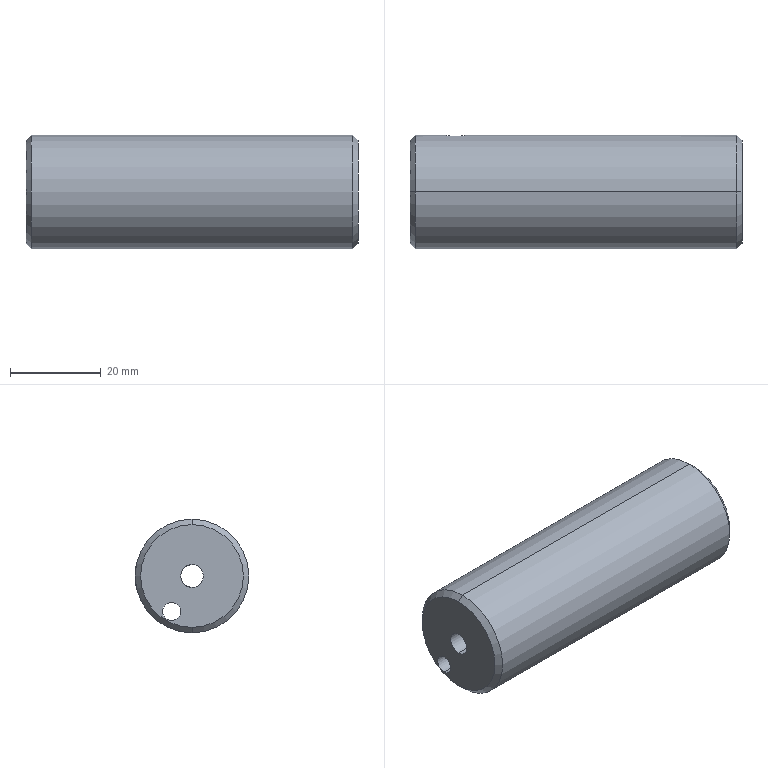Part | NX | features BREP 1 | 1 solid | 15 faces | box 73 x 25 x 25 mm | volume 33171 mm3 | cylinder 9 | cone 4 | plane 2 | commonest cylinder face diameters 5 x5 4 x2 25 x2
STEP:
#1=CARTESIAN_POINT('',(762.255,39.549,-64.084));
#2=VERTEX_POINT('',#1);
#3=CARTESIAN_POINT('',(763.455,39.549,-62.884));
#4=VERTEX_POINT('',#3);
#5=CARTESIAN_POINT('',(762.255,39.549,-64.084));
#6=DIRECTION('',(0.7071,0.,0.7071));
#7=VECTOR('',#6,1000.);
#8=LINE('',#5,#7);
#9=EDGE_CURVE('',#2,#4,#8,.T.);
#10=ORIENTED_EDGE('',*,*,#9,.T.);
#11=CARTESIAN_POINT('',(763.455,39.549,-40.284));
#12=VERTEX_POINT('',#11);
#13=CARTESIAN_POINT('',(763.455,39.549,-51.584));
#14=DIRECTION('',(1.,0.,0.));
#15=DIRECTION('',(0.,0.,1.));
#16=AXIS2_PLACEMENT_3D('',#13,#14,#15);
#17=CIRCLE('',#16,11.3);
#18=EDGE_CURVE('',#12,#4,#17,.T.);
#19=ORIENTED_EDGE('',*,*,#18,.F.);
#20=CARTESIAN_POINT('',(762.255,39.549,-39.084));
#21=VERTEX_POINT('',#20);
#22=CARTESIAN_POINT('',(762.255,39.549,-39.084));
#23=DIRECTION('',(0.7071,0.,-0.7071));
#24=VECTOR('',#23,1000.);
#25=LINE('',#22,#24);
#26=EDGE_CURVE('',#21,#12,#25,.T.);
#27=ORIENTED_EDGE('',*,*,#26,.F.);
#28=CARTESIAN_POINT('',(762.255,39.549,-51.584));
#29=DIRECTION('',(-1.,0.,0.));
#30=DIRECTION('',(0.,0.,1.));
#31=AXIS2_PLACEMENT_3D('',#28,#29,#30);
#32=CIRCLE('',#31,12.5);
#33=EDGE_CURVE('',#2,#21,#32,.T.);
#34=ORIENTED_EDGE('',*,*,#33,.F.);
#35=EDGE_LOOP('',(#10,#19,#27,#34));
#36=FACE_BOUND('',#35,.T.);
#37=CARTESIAN_POINT('',(762.255,39.549,-51.584));
#38=DIRECTION('',(-1.,0.,0.));
#39=DIRECTION('',(0.,0.,-1.));
#40=AXIS2_PLACEMENT_3D('',#37,#38,#39);
#41=CONICAL_SURFACE('',#40,12.5,0.7854);
#42=ADVANCED_FACE('',(#36),#41,.T.);
#43=CARTESIAN_POINT('',(690.455,39.549,-40.284));
#44=VERTEX_POINT('',#43);
#45=CARTESIAN_POINT('',(691.655,39.549,-39.084));
#46=VERTEX_POINT('',#45);
#47=CARTESIAN_POINT('',(690.455,39.549,-40.284));
#48=DIRECTION('',(-0.7071,0.,-0.7071));
#49=VECTOR('',#48,1000.);
#50=LINE('',#47,#49);
#51=EDGE_CURVE('',#44,#46,#50,.F.);
#52=ORIENTED_EDGE('',*,*,#51,.F.);
#53=CARTESIAN_POINT('',(690.455,39.549,-62.884));
#54=VERTEX_POINT('',#53);
#55=CARTESIAN_POINT('',(690.455,39.549,-51.584));
#56=DIRECTION('',(-1.,0.,0.));
#57=DIRECTION('',(0.,0.,1.));
#58=AXIS2_PLACEMENT_3D('',#55,#56,#57);
#59=CIRCLE('',#58,11.3);
#60=EDGE_CURVE('',#54,#44,#59,.T.);
#61=ORIENTED_EDGE('',*,*,#60,.F.);
#62=CARTESIAN_POINT('',(691.655,39.549,-64.084));
#63=VERTEX_POINT('',#62);
#64=CARTESIAN_POINT('',(690.455,39.549,-62.884));
#65=DIRECTION('',(-0.7071,0.,0.7071));
#66=VECTOR('',#65,1000.);
#67=LINE('',#64,#66);
#68=EDGE_CURVE('',#54,#63,#67,.F.);
#69=ORIENTED_EDGE('',*,*,#68,.T.);
#70=CARTESIAN_POINT('',(691.655,39.549,-51.584));
#71=DIRECTION('',(1.,0.,0.));
#72=DIRECTION('',(0.,0.,1.));
#73=AXIS2_PLACEMENT_3D('',#70,#71,#72);
#74=CIRCLE('',#73,12.5);
#75=EDGE_CURVE('',#46,#63,#74,.T.);
#76=ORIENTED_EDGE('',*,*,#75,.F.);
#77=EDGE_LOOP('',(#52,#61,#69,#76));
#78=FACE_BOUND('',#77,.T.);
#79=CARTESIAN_POINT('',(690.455,39.549,-51.584));
#80=DIRECTION('',(1.,0.,0.));
#81=DIRECTION('',(0.,0.,1.));
#82=AXIS2_PLACEMENT_3D('',#79,#80,#81);
#83=CONICAL_SURFACE('',#82,11.3,0.7854);
#84=ADVANCED_FACE('',(#78),#83,.T.);
#85=CARTESIAN_POINT('',(697.955,42.049,-51.584));
#86=VERTEX_POINT('',#85);
#87=CARTESIAN_POINT('',(697.955,52.049,-51.584));
#88=VERTEX_POINT('',#87);
#89=CARTESIAN_POINT('',(697.955,52.049,-51.584));
#90=DIRECTION('',(0.,-1.,0.));
#91=VECTOR('',#90,1000.);
#92=LINE('',#89,#91);
#93=EDGE_CURVE('',#86,#88,#92,.F.);
#94=ORIENTED_EDGE('',*,*,#93,.T.);
#95=CARTESIAN_POINT('',(702.955,52.049,-51.584));
#96=VERTEX_POINT('',#95);
#97=CARTESIAN_POINT('',(697.955,52.049,-51.584));
#98=CARTESIAN_POINT('',(697.955,52.049,-50.921));
#99=CARTESIAN_POINT('',(698.497,51.924,-49.629));
#100=CARTESIAN_POINT('',(700.452,51.733,-48.811));
#101=CARTESIAN_POINT('',(702.413,51.924,-49.627));
#102=CARTESIAN_POINT('',(702.955,52.049,-50.921));
#103=CARTESIAN_POINT('',(702.955,52.049,-51.584));
#104=B_SPLINE_CURVE_WITH_KNOTS('',3,(#97,#98,#99,#100,#101,#102,#103),.UNSPECIFIED.,.F.,.F.,(4,1,1,1,4),(0.,0.001958,0.003917,0.005875,0.007834),.UNSPECIFIED.);
#105=EDGE_CURVE('',#88,#96,#104,.T.);
#106=ORIENTED_EDGE('',*,*,#105,.T.);
#107=CARTESIAN_POINT('',(702.955,42.049,-51.584));
#108=VERTEX_POINT('',#107);
#109=CARTESIAN_POINT('',(702.955,52.049,-51.584));
#110=DIRECTION('',(0.,-1.,0.));
#111=VECTOR('',#110,1000.);
#112=LINE('',#109,#111);
#113=EDGE_CURVE('',#108,#96,#112,.F.);
#114=ORIENTED_EDGE('',*,*,#113,.F.);
#115=CARTESIAN_POINT('',(700.455,39.549,-49.084));
#116=VERTEX_POINT('',#115);
#117=CARTESIAN_POINT('',(700.455,39.549,-49.084));
#118=CARTESIAN_POINT('',(701.92,41.014,-49.084));
#119=CARTESIAN_POINT('',(702.955,42.049,-50.119));
#120=CARTESIAN_POINT('',(702.955,42.049,-51.584));
#121=(BOUNDED_CURVE()B_SPLINE_CURVE(3,(#117,#118,#119,#120),.UNSPECIFIED.,.F.,.F.)B_SPLINE_CURVE_WITH_KNOTS((4,4),(0.,1.),.PIECEWISE_BEZIER_KNOTS.)CURVE()GEOMETRIC_REPRESENTATION_ITEM()RATIONAL_B_SPLINE_CURVE((1.,0.8047,0.8047,1.))REPRESENTATION_ITEM(''));
#122=EDGE_CURVE('',#116,#108,#121,.T.);
#123=ORIENTED_EDGE('',*,*,#122,.F.);
#124=CARTESIAN_POINT('',(697.955,42.049,-51.584));
#125=CARTESIAN_POINT('',(697.955,42.049,-50.119));
#126=CARTESIAN_POINT('',(698.991,41.014,-49.084));
#127=CARTESIAN_POINT('',(700.455,39.549,-49.084));
#128=(BOUNDED_CURVE()B_SPLINE_CURVE(3,(#124,#125,#126,#127),.UNSPECIFIED.,.F.,.F.)B_SPLINE_CURVE_WITH_KNOTS((4,4),(0.,1.),.PIECEWISE_BEZIER_KNOTS.)CURVE()GEOMETRIC_REPRESENTATION_ITEM()RATIONAL_B_SPLINE_CURVE((1.,0.8047,0.8047,1.))REPRESENTATION_ITEM(''));
#129=EDGE_CURVE('',#86,#116,#128,.T.);
#130=ORIENTED_EDGE('',*,*,#129,.F.);
#131=EDGE_LOOP('',(#94,#106,#114,#123,#130));
#132=FACE_BOUND('',#131,.T.);
#133=CARTESIAN_POINT('',(700.455,52.049,-51.584));
#134=DIRECTION('',(0.,-1.,0.));
#135=DIRECTION('',(-1.,0.,0.));
#136=AXIS2_PLACEMENT_3D('',#133,#134,#135);
#137=CYLINDRICAL_SURFACE('',#136,2.5);
#138=ADVANCED_FACE('',(#132),#137,.F.);
#139=CARTESIAN_POINT('',(690.455,44.049,-61.378));
#140=VERTEX_POINT('',#139);
#141=CARTESIAN_POINT('',(763.455,44.049,-61.378));
#142=VERTEX_POINT('',#141);
#143=CARTESIAN_POINT('',(763.455,44.049,-61.378));
#144=DIRECTION('',(1.,0.,0.));
#145=VECTOR('',#144,1000.);
#146=LINE('',#143,#145);
#147=EDGE_CURVE('',#140,#142,#146,.T.);
#148=ORIENTED_EDGE('',*,*,#147,.T.);
#149=CARTESIAN_POINT('',(763.455,44.049,-57.378));
#150=VERTEX_POINT('',#149);
#151=CARTESIAN_POINT('',(763.455,44.049,-59.378));
#152=DIRECTION('',(-1.,0.,0.));
#153=DIRECTION('',(0.,0.,1.));
#154=AXIS2_PLACEMENT_3D('',#151,#152,#153);
#155=CIRCLE('',#154,2.);
#156=EDGE_CURVE('',#150,#142,#155,.T.);
#157=ORIENTED_EDGE('',*,*,#156,.F.);
#158=CARTESIAN_POINT('',(690.455,44.049,-57.378));
#159=VERTEX_POINT('',#158);
#160=CARTESIAN_POINT('',(763.455,44.049,-57.378));
#161=DIRECTION('',(1.,0.,0.));
#162=VECTOR('',#161,1000.);
#163=LINE('',#160,#162);
#164=EDGE_CURVE('',#159,#150,#163,.T.);
#165=ORIENTED_EDGE('',*,*,#164,.F.);
#166=CARTESIAN_POINT('',(690.455,44.049,-59.378));
#167=DIRECTION('',(-1.,0.,0.));
#168=DIRECTION('',(0.,0.,1.));
#169=AXIS2_PLACEMENT_3D('',#166,#167,#168);
#170=CIRCLE('',#169,2.);
#171=EDGE_CURVE('',#159,#140,#170,.T.);
#172=ORIENTED_EDGE('',*,*,#171,.T.);
#173=EDGE_LOOP('',(#148,#157,#165,#172));
#174=FACE_BOUND('',#173,.T.);
#175=CARTESIAN_POINT('',(763.455,44.049,-59.378));
#176=DIRECTION('',(-1.,0.,0.));
#177=DIRECTION('',(0.,0.,-1.));
#178=AXIS2_PLACEMENT_3D('',#175,#176,#177);
#179=CYLINDRICAL_SURFACE('',#178,2.);
#180=ADVANCED_FACE('',(#174),#179,.F.);
#181=CARTESIAN_POINT('',(763.455,39.549,-54.084));
#182=VERTEX_POINT('',#181);
#183=CARTESIAN_POINT('',(763.455,39.549,-49.084));
#184=VERTEX_POINT('',#183);
#185=CARTESIAN_POINT('',(763.455,39.549,-51.584));
#186=DIRECTION('',(-1.,0.,0.));
#187=DIRECTION('',(0.,0.,1.));
#188=AXIS2_PLACEMENT_3D('',#185,#186,#187);
#189=CIRCLE('',#188,2.5);
#190=EDGE_CURVE('',#182,#184,#189,.T.);
#191=ORIENTED_EDGE('',*,*,#190,.T.);
#192=CARTESIAN_POINT('',(763.455,39.549,-51.584));
#193=DIRECTION('',(-1.,0.,0.));
#194=DIRECTION('',(0.,0.,1.));
#195=AXIS2_PLACEMENT_3D('',#192,#193,#194);
#196=CIRCLE('',#195,2.5);
#197=EDGE_CURVE('',#184,#182,#196,.T.);
#198=ORIENTED_EDGE('',*,*,#197,.T.);
#199=EDGE_LOOP('',(#191,#198));
#200=FACE_BOUND('',#199,.T.);
#201=ORIENTED_EDGE('',*,*,#156,.T.);
#202=CARTESIAN_POINT('',(763.455,44.049,-59.378));
#203=DIRECTION('',(-1.,0.,0.));
#204=DIRECTION('',(0.,0.,1.));
#205=AXIS2_PLACEMENT_3D('',#202,#203,#204);
#206=CIRCLE('',#205,2.);
#207=EDGE_CURVE('',#142,#150,#206,.T.);
#208=ORIENTED_EDGE('',*,*,#207,.T.);
#209=EDGE_LOOP('',(#201,#208));
#210=FACE_BOUND('',#209,.T.);
#211=ORIENTED_EDGE('',*,*,#18,.T.);
#212=CARTESIAN_POINT('',(763.455,39.549,-51.584));
#213=DIRECTION('',(1.,0.,0.));
#214=DIRECTION('',(0.,0.,1.));
#215=AXIS2_PLACEMENT_3D('',#212,#213,#214);
#216=CIRCLE('',#215,11.3);
#217=EDGE_CURVE('',#4,#12,#216,.T.);
#218=ORIENTED_EDGE('',*,*,#217,.T.);
#219=EDGE_LOOP('',(#211,#218));
#220=FACE_BOUND('',#219,.T.);
#221=CARTESIAN_POINT('',(763.455,39.549,-51.584));
#222=DIRECTION('',(-1.,0.,0.));
#223=DIRECTION('',(0.,0.,-1.));
#224=AXIS2_PLACEMENT_3D('',#221,#222,#223);
#225=PLANE('',#224);
#226=ADVANCED_FACE('',(#200,#210,#220),#225,.F.);
#227=CARTESIAN_POINT('',(690.455,39.549,-54.084));
#228=VERTEX_POINT('',#227);
#229=CARTESIAN_POINT('',(690.455,39.549,-49.084));
#230=VERTEX_POINT('',#229);
#231=CARTESIAN_POINT('',(690.455,39.549,-51.584));
#232=DIRECTION('',(-1.,0.,0.));
#233=DIRECTION('',(0.,0.,1.));
#234=AXIS2_PLACEMENT_3D('',#231,#232,#233);
#235=CIRCLE('',#234,2.5);
#236=EDGE_CURVE('',#228,#230,#235,.T.);
#237=ORIENTED_EDGE('',*,*,#236,.F.);
#238=CARTESIAN_POINT('',(690.455,39.549,-51.584));
#239=DIRECTION('',(-1.,0.,0.));
#240=DIRECTION('',(0.,0.,1.));
#241=AXIS2_PLACEMENT_3D('',#238,#239,#240);
#242=CIRCLE('',#241,2.5);
#243=EDGE_CURVE('',#230,#228,#242,.T.);
#244=ORIENTED_EDGE('',*,*,#243,.F.);
#245=EDGE_LOOP('',(#237,#244));
#246=FACE_BOUND('',#245,.T.);
#247=ORIENTED_EDGE('',*,*,#171,.F.);
#248=CARTESIAN_POINT('',(690.455,44.049,-59.378));
#249=DIRECTION('',(-1.,0.,0.));
#250=DIRECTION('',(0.,0.,1.));
#251=AXIS2_PLACEMENT_3D('',#248,#249,#250);
#252=CIRCLE('',#251,2.);
#253=EDGE_CURVE('',#140,#159,#252,.T.);
#254=ORIENTED_EDGE('',*,*,#253,.F.);
#255=EDGE_LOOP('',(#247,#254));
#256=FACE_BOUND('',#255,.T.);
#257=ORIENTED_EDGE('',*,*,#60,.T.);
#258=CARTESIAN_POINT('',(690.455,39.549,-51.584));
#259=DIRECTION('',(-1.,0.,0.));
#260=DIRECTION('',(0.,0.,1.));
#261=AXIS2_PLACEMENT_3D('',#258,#259,#260);
#262=CIRCLE('',#261,11.3);
#263=EDGE_CURVE('',#44,#54,#262,.T.);
#264=ORIENTED_EDGE('',*,*,#263,.T.);
#265=EDGE_LOOP('',(#257,#264));
#266=FACE_BOUND('',#265,.T.);
#267=CARTESIAN_POINT('',(690.455,39.549,-51.584));
#268=DIRECTION('',(-1.,0.,0.));
#269=DIRECTION('',(0.,0.,-1.));
#270=AXIS2_PLACEMENT_3D('',#267,#268,#269);
#271=PLANE('',#270);
#272=ADVANCED_FACE('',(#246,#256,#266),#271,.T.);
#273=CARTESIAN_POINT('',(690.455,39.549,-49.084));
#274=DIRECTION('',(-1.,0.,0.));
#275=VECTOR('',#274,1000.);
#276=LINE('',#273,#275);
#277=EDGE_CURVE('',#116,#184,#276,.F.);
#278=ORIENTED_EDGE('',*,*,#277,.F.);
#279=ORIENTED_EDGE('',*,*,#122,.T.);
#280=CARTESIAN_POINT('',(700.455,39.549,-54.084));
#281=VERTEX_POINT('',#280);
#282=CARTESIAN_POINT('',(702.955,42.049,-51.584));
#283=CARTESIAN_POINT('',(702.955,42.049,-53.048));
#284=CARTESIAN_POINT('',(701.92,41.014,-54.084));
#285=CARTESIAN_POINT('',(700.455,39.549,-54.084));
#286=(BOUNDED_CURVE()B_SPLINE_CURVE(3,(#282,#283,#284,#285),.UNSPECIFIED.,.F.,.F.)B_SPLINE_CURVE_WITH_KNOTS((4,4),(0.,1.),.PIECEWISE_BEZIER_KNOTS.)CURVE()GEOMETRIC_REPRESENTATION_ITEM()RATIONAL_B_SPLINE_CURVE((1.,0.8047,0.8047,1.))REPRESENTATION_ITEM(''));
#287=EDGE_CURVE('',#108,#281,#286,.T.);
#288=ORIENTED_EDGE('',*,*,#287,.T.);
#289=CARTESIAN_POINT('',(690.455,39.549,-54.084));
#290=DIRECTION('',(-1.,0.,0.));
#291=VECTOR('',#290,1000.);
#292=LINE('',#289,#291);
#293=EDGE_CURVE('',#281,#182,#292,.F.);
#294=ORIENTED_EDGE('',*,*,#293,.T.);
#295=ORIENTED_EDGE('',*,*,#197,.F.);
#296=EDGE_LOOP('',(#278,#279,#288,#294,#295));
#297=FACE_BOUND('',#296,.T.);
#298=CARTESIAN_POINT('',(690.455,39.549,-51.584));
#299=DIRECTION('',(1.,0.,0.));
#300=DIRECTION('',(0.,0.,1.));
#301=AXIS2_PLACEMENT_3D('',#298,#299,#300);
#302=CYLINDRICAL_SURFACE('',#301,2.5);
#303=ADVANCED_FACE('',(#297),#302,.F.);
#304=CARTESIAN_POINT('',(690.455,39.549,-39.084));
#305=DIRECTION('',(-1.,0.,0.));
#306=VECTOR('',#305,1000.);
#307=LINE('',#304,#306);
#308=EDGE_CURVE('',#46,#21,#307,.F.);
#309=ORIENTED_EDGE('',*,*,#308,.F.);
#310=ORIENTED_EDGE('',*,*,#75,.T.);
#311=CARTESIAN_POINT('',(690.455,39.549,-64.084));
#312=DIRECTION('',(-1.,0.,0.));
#313=VECTOR('',#312,1000.);
#314=LINE('',#311,#313);
#315=EDGE_CURVE('',#63,#2,#314,.F.);
#316=ORIENTED_EDGE('',*,*,#315,.T.);
#317=ORIENTED_EDGE('',*,*,#33,.T.);
#318=EDGE_LOOP('',(#309,#310,#316,#317));
#319=FACE_BOUND('',#318,.T.);
#320=CARTESIAN_POINT('',(690.455,39.549,-51.584));
#321=DIRECTION('',(1.,0.,0.));
#322=DIRECTION('',(0.,0.,1.));
#323=AXIS2_PLACEMENT_3D('',#320,#321,#322);
#324=CYLINDRICAL_SURFACE('',#323,12.5);
#325=ADVANCED_FACE('',(#319),#324,.T.);
#326=CARTESIAN_POINT('',(702.955,52.049,-51.584));
#327=CARTESIAN_POINT('',(702.955,52.049,-52.246));
#328=CARTESIAN_POINT('',(702.413,51.924,-53.538));
#329=CARTESIAN_POINT('',(700.458,51.733,-54.356));
#330=CARTESIAN_POINT('',(698.497,51.924,-53.54));
#331=CARTESIAN_POINT('',(697.955,52.049,-52.246));
#332=CARTESIAN_POINT('',(697.955,52.049,-51.584));
#333=B_SPLINE_CURVE_WITH_KNOTS('',3,(#326,#327,#328,#329,#330,#331,#332),.UNSPECIFIED.,.F.,.F.,(4,1,1,1,4),(0.,0.001958,0.003917,0.005875,0.007834),.UNSPECIFIED.);
#334=EDGE_CURVE('',#96,#88,#333,.T.);
#335=ORIENTED_EDGE('',*,*,#334,.F.);
#336=ORIENTED_EDGE('',*,*,#105,.F.);
#337=EDGE_LOOP('',(#335,#336));
#338=FACE_BOUND('',#337,.T.);
#339=CARTESIAN_POINT('',(691.655,39.549,-51.584));
#340=DIRECTION('',(1.,0.,0.));
#341=DIRECTION('',(0.,0.,1.));
#342=AXIS2_PLACEMENT_3D('',#339,#340,#341);
#343=CIRCLE('',#342,12.5);
#344=EDGE_CURVE('',#63,#46,#343,.T.);
#345=ORIENTED_EDGE('',*,*,#344,.T.);
#346=ORIENTED_EDGE('',*,*,#308,.T.);
#347=CARTESIAN_POINT('',(762.255,39.549,-51.584));
#348=DIRECTION('',(-1.,0.,0.));
#349=DIRECTION('',(0.,0.,1.));
#350=AXIS2_PLACEMENT_3D('',#347,#348,#349);
#351=CIRCLE('',#350,12.5);
#352=EDGE_CURVE('',#21,#2,#351,.T.);
#353=ORIENTED_EDGE('',*,*,#352,.T.);
#354=ORIENTED_EDGE('',*,*,#315,.F.);
#355=EDGE_LOOP('',(#345,#346,#353,#354));
#356=FACE_BOUND('',#355,.T.);
#357=CARTESIAN_POINT('',(690.455,39.549,-51.584));
#358=DIRECTION('',(1.,0.,0.));
#359=DIRECTION('',(0.,0.,1.));
#360=AXIS2_PLACEMENT_3D('',#357,#358,#359);
#361=CYLINDRICAL_SURFACE('',#360,12.5);
#362=ADVANCED_FACE('',(#338,#356),#361,.T.);
#363=CARTESIAN_POINT('',(690.455,39.549,-49.084));
#364=DIRECTION('',(-1.,0.,0.));
#365=VECTOR('',#364,1000.);
#366=LINE('',#363,#365);
#367=EDGE_CURVE('',#230,#116,#366,.F.);
#368=ORIENTED_EDGE('',*,*,#367,.F.);
#369=ORIENTED_EDGE('',*,*,#243,.T.);
#370=CARTESIAN_POINT('',(690.455,39.549,-54.084));
#371=DIRECTION('',(-1.,0.,0.));
#372=VECTOR('',#371,1000.);
#373=LINE('',#370,#372);
#374=EDGE_CURVE('',#228,#281,#373,.F.);
#375=ORIENTED_EDGE('',*,*,#374,.T.);
#376=CARTESIAN_POINT('',(700.455,39.549,-54.084));
#377=CARTESIAN_POINT('',(698.991,41.014,-54.084));
#378=CARTESIAN_POINT('',(697.955,42.049,-53.048));
#379=CARTESIAN_POINT('',(697.955,42.049,-51.584));
#380=(BOUNDED_CURVE()B_SPLINE_CURVE(3,(#376,#377,#378,#379),.UNSPECIFIED.,.F.,.F.)B_SPLINE_CURVE_WITH_KNOTS((4,4),(0.,1.),.PIECEWISE_BEZIER_KNOTS.)CURVE()GEOMETRIC_REPRESENTATION_ITEM()RATIONAL_B_SPLINE_CURVE((1.,0.8047,0.8047,1.))REPRESENTATION_ITEM(''));
#381=EDGE_CURVE('',#281,#86,#380,.T.);
#382=ORIENTED_EDGE('',*,*,#381,.T.);
#383=ORIENTED_EDGE('',*,*,#129,.T.);
#384=EDGE_LOOP('',(#368,#369,#375,#382,#383));
#385=FACE_BOUND('',#384,.T.);
#386=CARTESIAN_POINT('',(690.455,39.549,-51.584));
#387=DIRECTION('',(1.,0.,0.));
#388=DIRECTION('',(0.,0.,1.));
#389=AXIS2_PLACEMENT_3D('',#386,#387,#388);
#390=CYLINDRICAL_SURFACE('',#389,2.5);
#391=ADVANCED_FACE('',(#385),#390,.F.);
#392=ORIENTED_EDGE('',*,*,#236,.T.);
#393=ORIENTED_EDGE('',*,*,#367,.T.);
#394=ORIENTED_EDGE('',*,*,#277,.T.);
#395=ORIENTED_EDGE('',*,*,#190,.F.);
#396=ORIENTED_EDGE('',*,*,#293,.F.);
#397=ORIENTED_EDGE('',*,*,#374,.F.);
#398=EDGE_LOOP('',(#392,#393,#394,#395,#396,#397));
#399=FACE_BOUND('',#398,.T.);
#400=CARTESIAN_POINT('',(690.455,39.549,-51.584));
#401=DIRECTION('',(1.,0.,0.));
#402=DIRECTION('',(0.,0.,1.));
#403=AXIS2_PLACEMENT_3D('',#400,#401,#402);
#404=CYLINDRICAL_SURFACE('',#403,2.5);
#405=ADVANCED_FACE('',(#399),#404,.F.);
#406=ORIENTED_EDGE('',*,*,#207,.F.);
#407=ORIENTED_EDGE('',*,*,#147,.F.);
#408=ORIENTED_EDGE('',*,*,#253,.T.);
#409=ORIENTED_EDGE('',*,*,#164,.T.);
#410=EDGE_LOOP('',(#406,#407,#408,#409));
#411=FACE_BOUND('',#410,.T.);
#412=CARTESIAN_POINT('',(763.455,44.049,-59.378));
#413=DIRECTION('',(-1.,0.,0.));
#414=DIRECTION('',(0.,0.,-1.));
#415=AXIS2_PLACEMENT_3D('',#412,#413,#414);
#416=CYLINDRICAL_SURFACE('',#415,2.);
#417=ADVANCED_FACE('',(#411),#416,.F.);
#418=ORIENTED_EDGE('',*,*,#334,.T.);
#419=ORIENTED_EDGE('',*,*,#93,.F.);
#420=ORIENTED_EDGE('',*,*,#381,.F.);
#421=ORIENTED_EDGE('',*,*,#287,.F.);
#422=ORIENTED_EDGE('',*,*,#113,.T.);
#423=EDGE_LOOP('',(#418,#419,#420,#421,#422));
#424=FACE_BOUND('',#423,.T.);
#425=CARTESIAN_POINT('',(700.455,52.049,-51.584));
#426=DIRECTION('',(0.,-1.,0.));
#427=DIRECTION('',(-1.,0.,0.));
#428=AXIS2_PLACEMENT_3D('',#425,#426,#427);
#429=CYLINDRICAL_SURFACE('',#428,2.5);
#430=ADVANCED_FACE('',(#424),#429,.F.);
#431=ORIENTED_EDGE('',*,*,#263,.F.);
#432=ORIENTED_EDGE('',*,*,#51,.T.);
#433=ORIENTED_EDGE('',*,*,#344,.F.);
#434=ORIENTED_EDGE('',*,*,#68,.F.);
#435=EDGE_LOOP('',(#431,#432,#433,#434));
#436=FACE_BOUND('',#435,.T.);
#437=CARTESIAN_POINT('',(690.455,39.549,-51.584));
#438=DIRECTION('',(1.,0.,0.));
#439=DIRECTION('',(0.,0.,1.));
#440=AXIS2_PLACEMENT_3D('',#437,#438,#439);
#441=CONICAL_SURFACE('',#440,11.3,0.7854);
#442=ADVANCED_FACE('',(#436),#441,.T.);
#443=ORIENTED_EDGE('',*,*,#217,.F.);
#444=ORIENTED_EDGE('',*,*,#9,.F.);
#445=ORIENTED_EDGE('',*,*,#352,.F.);
#446=ORIENTED_EDGE('',*,*,#26,.T.);
#447=EDGE_LOOP('',(#443,#444,#445,#446));
#448=FACE_BOUND('',#447,.T.);
#449=CARTESIAN_POINT('',(762.255,39.549,-51.584));
#450=DIRECTION('',(-1.,0.,0.));
#451=DIRECTION('',(0.,0.,-1.));
#452=AXIS2_PLACEMENT_3D('',#449,#450,#451);
#453=CONICAL_SURFACE('',#452,12.5,0.7854);
#454=ADVANCED_FACE('',(#448),#453,.T.);
#455=CLOSED_SHELL('',(#42,#84,#138,#180,#226,#272,#303,#325,#362,#391,#405,#417,#430,#442,#454));
#456=MANIFOLD_SOLID_BREP('',#455);
#457=(LENGTH_UNIT()NAMED_UNIT(*)SI_UNIT(.MILLI.,.METRE.));
#458=UNCERTAINTY_MEASURE_WITH_UNIT(LENGTH_MEASURE(0.0508),#457,'','');
#459=(NAMED_UNIT(*)PLANE_ANGLE_UNIT()SI_UNIT($,.RADIAN.));
#460=(NAMED_UNIT(*)SI_UNIT($,.STERADIAN.)SOLID_ANGLE_UNIT());
#461=(GEOMETRIC_REPRESENTATION_CONTEXT(3)GLOBAL_UNCERTAINTY_ASSIGNED_CONTEXT((#458))GLOBAL_UNIT_ASSIGNED_CONTEXT((#457,#459,#460))REPRESENTATION_CONTEXT('',''));
#462=ADVANCED_BREP_SHAPE_REPRESENTATION('',(#456),#461);